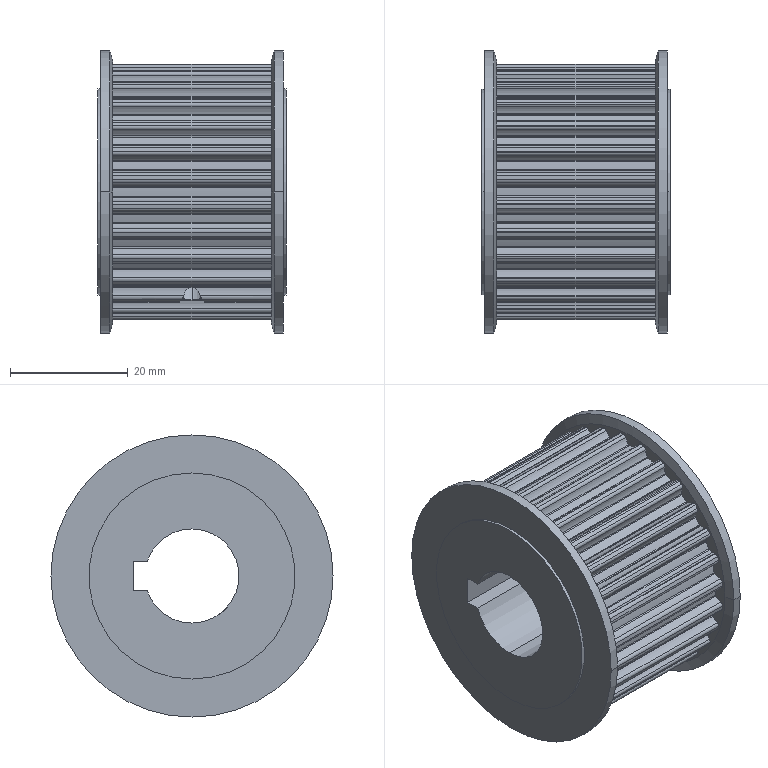Part | SolidWorks | features RevCut 8, ICE 5, Revolution 3, Fillet 2, CirPattern 1 | 1 solid | 290 faces | box 32 x 47.9 x 47.9 mm | volume 37659 mm3 | cylinder 277 | plane 9 | cone 4 | commonest cylinder face diameters 1.1 x72 0.5 x67 6.55 x64 40.06 x30 43.6 x29 4.3 x4